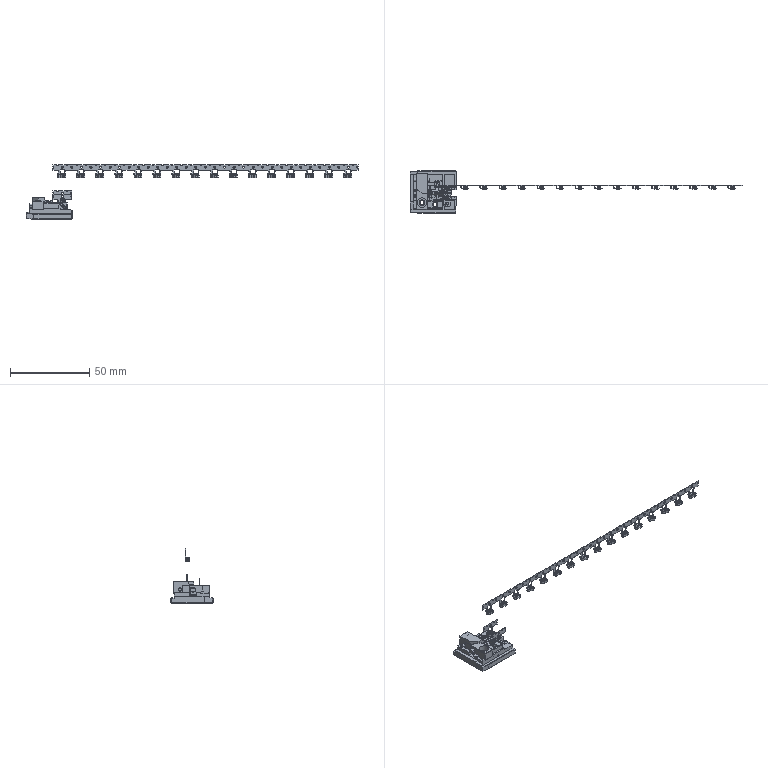Part | NX | 11 solids | 3907 faces | volume 5183 mm3 | plane 2299 | cylinder 1224 | torus 254 | spline 54 | sphere 48 | cone 28 | commonest cylinder face diameters 0.3 x288 0.2 x206 0.7 x98 1.3 x93 0.5 x91 0.4 x85